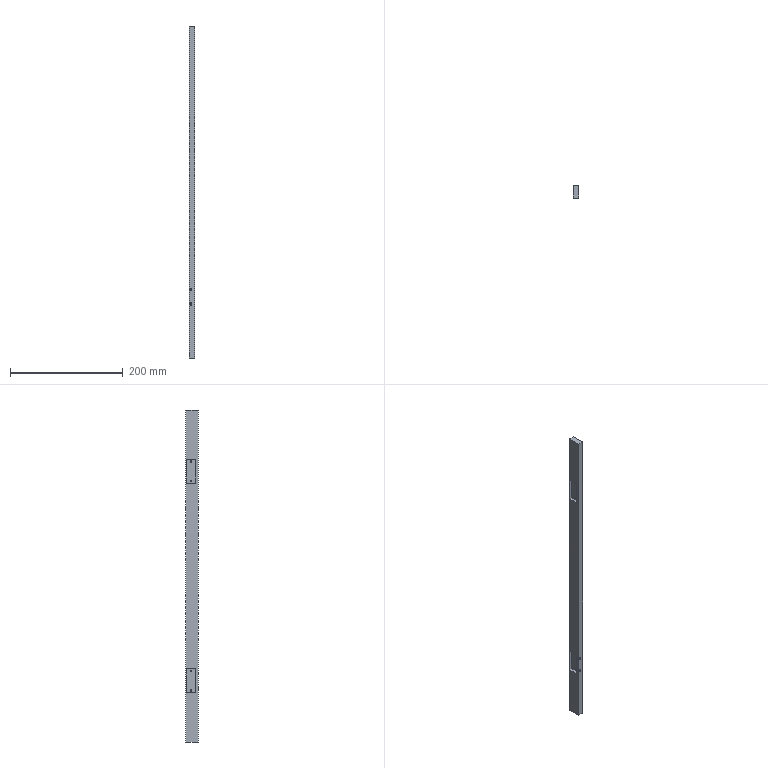Part | SolidWorks | features 3DProfileFeature 2, HoleWzd 2, MirrorPattern 2, Cut 1, Extrusion 1 | 1 solid | 46 faces | box 10 x 23 x 590 mm | volume 128132 mm3 | cylinder 24 | plane 22 | commonest cylinder face diameters 2.9 x8 5.5 x8 2.4 x4 4.4 x4
STEP:
#1=CARTESIAN_POINT('',(-2.5,2.4,-170.8));
#2=VERTEX_POINT('',#1);
#3=CARTESIAN_POINT('',(-2.5,2.4,-175.2));
#4=VERTEX_POINT('',#3);
#5=CARTESIAN_POINT('',(-2.5,2.4,-173.));
#6=DIRECTION('',(0.,-1.,0.));
#7=DIRECTION('',(0.,0.,-1.));
#8=AXIS2_PLACEMENT_3D('',#5,#6,#7);
#9=CIRCLE('',#8,2.2);
#10=EDGE_CURVE('',#2,#4,#9,.T.);
#11=ORIENTED_EDGE('',*,*,#10,.F.);
#12=CARTESIAN_POINT('',(-2.5,0.,-170.8));
#13=VERTEX_POINT('',#12);
#14=CARTESIAN_POINT('',(-2.5,0.,-170.8));
#15=DIRECTION('',(0.,-1.,0.));
#16=VECTOR('',#15,1000.);
#17=LINE('',#14,#16);
#18=EDGE_CURVE('',#2,#13,#17,.T.);
#19=ORIENTED_EDGE('',*,*,#18,.T.);
#20=CARTESIAN_POINT('',(-2.5,0.,-175.2));
#21=VERTEX_POINT('',#20);
#22=CARTESIAN_POINT('',(-2.5,0.,-173.));
#23=DIRECTION('',(0.,-1.,0.));
#24=DIRECTION('',(0.,0.,-1.));
#25=AXIS2_PLACEMENT_3D('',#22,#23,#24);
#26=CIRCLE('',#25,2.2);
#27=EDGE_CURVE('',#13,#21,#26,.T.);
#28=ORIENTED_EDGE('',*,*,#27,.T.);
#29=CARTESIAN_POINT('',(-2.5,0.,-175.2));
#30=DIRECTION('',(0.,-1.,0.));
#31=VECTOR('',#30,1000.);
#32=LINE('',#29,#31);
#33=EDGE_CURVE('',#4,#21,#32,.T.);
#34=ORIENTED_EDGE('',*,*,#33,.F.);
#35=EDGE_LOOP('',(#11,#19,#28,#34));
#36=FACE_OUTER_BOUND('',#35,.T.);
#37=CARTESIAN_POINT('',(-2.5,0.,-173.));
#38=DIRECTION('',(0.,-1.,0.));
#39=DIRECTION('',(0.,0.,-1.));
#40=AXIS2_PLACEMENT_3D('',#37,#38,#39);
#41=CYLINDRICAL_SURFACE('',#40,2.2);
#42=ADVANCED_FACE('',(#36),#41,.F.);
#43=CARTESIAN_POINT('',(-2.5,5.,-171.8));
#44=VERTEX_POINT('',#43);
#45=CARTESIAN_POINT('',(-2.5,5.,-174.2));
#46=VERTEX_POINT('',#45);
#47=CARTESIAN_POINT('',(-2.5,5.,-173.));
#48=DIRECTION('',(0.,-1.,0.));
#49=DIRECTION('',(0.,0.,-1.));
#50=AXIS2_PLACEMENT_3D('',#47,#48,#49);
#51=CIRCLE('',#50,1.2);
#52=EDGE_CURVE('',#44,#46,#51,.T.);
#53=ORIENTED_EDGE('',*,*,#52,.F.);
#54=CARTESIAN_POINT('',(-2.5,2.4,-171.8));
#55=VERTEX_POINT('',#54);
#56=CARTESIAN_POINT('',(-2.5,0.,-171.8));
#57=DIRECTION('',(0.,-1.,0.));
#58=VECTOR('',#57,1000.);
#59=LINE('',#56,#58);
#60=EDGE_CURVE('',#44,#55,#59,.T.);
#61=ORIENTED_EDGE('',*,*,#60,.T.);
#62=CARTESIAN_POINT('',(-2.5,2.4,-174.2));
#63=VERTEX_POINT('',#62);
#64=CARTESIAN_POINT('',(-2.5,2.4,-173.));
#65=DIRECTION('',(0.,-1.,0.));
#66=DIRECTION('',(0.,0.,-1.));
#67=AXIS2_PLACEMENT_3D('',#64,#65,#66);
#68=CIRCLE('',#67,1.2);
#69=EDGE_CURVE('',#55,#63,#68,.T.);
#70=ORIENTED_EDGE('',*,*,#69,.T.);
#71=CARTESIAN_POINT('',(-2.5,0.,-174.2));
#72=DIRECTION('',(0.,-1.,0.));
#73=VECTOR('',#72,1000.);
#74=LINE('',#71,#73);
#75=EDGE_CURVE('',#46,#63,#74,.T.);
#76=ORIENTED_EDGE('',*,*,#75,.F.);
#77=EDGE_LOOP('',(#53,#61,#70,#76));
#78=FACE_OUTER_BOUND('',#77,.T.);
#79=CARTESIAN_POINT('',(-2.5,0.,-173.));
#80=DIRECTION('',(0.,-1.,0.));
#81=DIRECTION('',(0.,0.,-1.));
#82=AXIS2_PLACEMENT_3D('',#79,#80,#81);
#83=CYLINDRICAL_SURFACE('',#82,1.2);
#84=ADVANCED_FACE('',(#78),#83,.F.);
#85=CARTESIAN_POINT('',(-2.5,2.4,-196.8));
#86=VERTEX_POINT('',#85);
#87=CARTESIAN_POINT('',(-2.5,2.4,-201.2));
#88=VERTEX_POINT('',#87);
#89=CARTESIAN_POINT('',(-2.5,2.4,-199.));
#90=DIRECTION('',(0.,-1.,0.));
#91=DIRECTION('',(0.,0.,-1.));
#92=AXIS2_PLACEMENT_3D('',#89,#90,#91);
#93=CIRCLE('',#92,2.2);
#94=EDGE_CURVE('',#86,#88,#93,.T.);
#95=ORIENTED_EDGE('',*,*,#94,.F.);
#96=CARTESIAN_POINT('',(-2.5,0.,-196.8));
#97=VERTEX_POINT('',#96);
#98=CARTESIAN_POINT('',(-2.5,0.,-196.8));
#99=DIRECTION('',(0.,-1.,0.));
#100=VECTOR('',#99,1000.);
#101=LINE('',#98,#100);
#102=EDGE_CURVE('',#86,#97,#101,.T.);
#103=ORIENTED_EDGE('',*,*,#102,.T.);
#104=CARTESIAN_POINT('',(-2.5,0.,-201.2));
#105=VERTEX_POINT('',#104);
#106=CARTESIAN_POINT('',(-2.5,0.,-199.));
#107=DIRECTION('',(0.,-1.,0.));
#108=DIRECTION('',(0.,0.,-1.));
#109=AXIS2_PLACEMENT_3D('',#106,#107,#108);
#110=CIRCLE('',#109,2.2);
#111=EDGE_CURVE('',#97,#105,#110,.T.);
#112=ORIENTED_EDGE('',*,*,#111,.T.);
#113=CARTESIAN_POINT('',(-2.5,0.,-201.2));
#114=DIRECTION('',(0.,-1.,0.));
#115=VECTOR('',#114,1000.);
#116=LINE('',#113,#115);
#117=EDGE_CURVE('',#88,#105,#116,.T.);
#118=ORIENTED_EDGE('',*,*,#117,.F.);
#119=EDGE_LOOP('',(#95,#103,#112,#118));
#120=FACE_OUTER_BOUND('',#119,.T.);
#121=CARTESIAN_POINT('',(-2.5,0.,-199.));
#122=DIRECTION('',(0.,-1.,0.));
#123=DIRECTION('',(0.,0.,-1.));
#124=AXIS2_PLACEMENT_3D('',#121,#122,#123);
#125=CYLINDRICAL_SURFACE('',#124,2.2);
#126=ADVANCED_FACE('',(#120),#125,.F.);
#127=CARTESIAN_POINT('',(-2.5,5.,-197.8));
#128=VERTEX_POINT('',#127);
#129=CARTESIAN_POINT('',(-2.5,5.,-200.2));
#130=VERTEX_POINT('',#129);
#131=CARTESIAN_POINT('',(-2.5,5.,-199.));
#132=DIRECTION('',(0.,-1.,0.));
#133=DIRECTION('',(0.,0.,-1.));
#134=AXIS2_PLACEMENT_3D('',#131,#132,#133);
#135=CIRCLE('',#134,1.2);
#136=EDGE_CURVE('',#128,#130,#135,.T.);
#137=ORIENTED_EDGE('',*,*,#136,.F.);
#138=CARTESIAN_POINT('',(-2.5,2.4,-197.8));
#139=VERTEX_POINT('',#138);
#140=CARTESIAN_POINT('',(-2.5,0.,-197.8));
#141=DIRECTION('',(0.,-1.,0.));
#142=VECTOR('',#141,1000.);
#143=LINE('',#140,#142);
#144=EDGE_CURVE('',#128,#139,#143,.T.);
#145=ORIENTED_EDGE('',*,*,#144,.T.);
#146=CARTESIAN_POINT('',(-2.5,2.4,-200.2));
#147=VERTEX_POINT('',#146);
#148=CARTESIAN_POINT('',(-2.5,2.4,-199.));
#149=DIRECTION('',(0.,-1.,0.));
#150=DIRECTION('',(0.,0.,-1.));
#151=AXIS2_PLACEMENT_3D('',#148,#149,#150);
#152=CIRCLE('',#151,1.2);
#153=EDGE_CURVE('',#139,#147,#152,.T.);
#154=ORIENTED_EDGE('',*,*,#153,.T.);
#155=CARTESIAN_POINT('',(-2.5,0.,-200.2));
#156=DIRECTION('',(0.,-1.,0.));
#157=VECTOR('',#156,1000.);
#158=LINE('',#155,#157);
#159=EDGE_CURVE('',#130,#147,#158,.T.);
#160=ORIENTED_EDGE('',*,*,#159,.F.);
#161=EDGE_LOOP('',(#137,#145,#154,#160));
#162=FACE_OUTER_BOUND('',#161,.T.);
#163=CARTESIAN_POINT('',(-2.5,0.,-199.));
#164=DIRECTION('',(0.,-1.,0.));
#165=DIRECTION('',(0.,0.,-1.));
#166=AXIS2_PLACEMENT_3D('',#163,#164,#165);
#167=CYLINDRICAL_SURFACE('',#166,1.2);
#168=ADVANCED_FACE('',(#162),#167,.F.);
#169=CARTESIAN_POINT('',(2.1,13.5,-200.25));
#170=VERTEX_POINT('',#169);
#171=CARTESIAN_POINT('',(2.1,13.5,-205.75));
#172=VERTEX_POINT('',#171);
#173=CARTESIAN_POINT('',(2.1,13.5,-203.));
#174=DIRECTION('',(1.,0.,0.));
#175=DIRECTION('',(0.,0.,-1.));
#176=AXIS2_PLACEMENT_3D('',#173,#174,#175);
#177=CIRCLE('',#176,2.75);
#178=EDGE_CURVE('',#170,#172,#177,.T.);
#179=ORIENTED_EDGE('',*,*,#178,.F.);
#180=CARTESIAN_POINT('',(5.,13.5,-200.25));
#181=VERTEX_POINT('',#180);
#182=CARTESIAN_POINT('',(5.,13.5,-200.25));
#183=DIRECTION('',(1.,0.,0.));
#184=VECTOR('',#183,1000.);
#185=LINE('',#182,#184);
#186=EDGE_CURVE('',#170,#181,#185,.T.);
#187=ORIENTED_EDGE('',*,*,#186,.T.);
#188=CARTESIAN_POINT('',(5.,13.5,-205.75));
#189=VERTEX_POINT('',#188);
#190=CARTESIAN_POINT('',(5.,13.5,-203.));
#191=DIRECTION('',(1.,0.,0.));
#192=DIRECTION('',(0.,0.,-1.));
#193=AXIS2_PLACEMENT_3D('',#190,#191,#192);
#194=CIRCLE('',#193,2.75);
#195=EDGE_CURVE('',#181,#189,#194,.T.);
#196=ORIENTED_EDGE('',*,*,#195,.T.);
#197=CARTESIAN_POINT('',(5.,13.5,-205.75));
#198=DIRECTION('',(1.,0.,0.));
#199=VECTOR('',#198,1000.);
#200=LINE('',#197,#199);
#201=EDGE_CURVE('',#172,#189,#200,.T.);
#202=ORIENTED_EDGE('',*,*,#201,.F.);
#203=EDGE_LOOP('',(#179,#187,#196,#202));
#204=FACE_OUTER_BOUND('',#203,.T.);
#205=CARTESIAN_POINT('',(5.,13.5,-203.));
#206=DIRECTION('',(1.,0.,0.));
#207=DIRECTION('',(0.,0.,-1.));
#208=AXIS2_PLACEMENT_3D('',#205,#206,#207);
#209=CYLINDRICAL_SURFACE('',#208,2.75);
#210=ADVANCED_FACE('',(#204),#209,.F.);
#211=CARTESIAN_POINT('',(0.,13.5,-204.45));
#212=VERTEX_POINT('',#211);
#213=CARTESIAN_POINT('',(0.,13.5,-201.55));
#214=VERTEX_POINT('',#213);
#215=CARTESIAN_POINT('',(0.,13.5,-203.));
#216=DIRECTION('',(-1.,0.,0.));
#217=DIRECTION('',(0.,0.,-1.));
#218=AXIS2_PLACEMENT_3D('',#215,#216,#217);
#219=CIRCLE('',#218,1.45);
#220=EDGE_CURVE('',#212,#214,#219,.T.);
#221=ORIENTED_EDGE('',*,*,#220,.T.);
#222=CARTESIAN_POINT('',(2.1,13.5,-201.55));
#223=VERTEX_POINT('',#222);
#224=CARTESIAN_POINT('',(5.,13.5,-201.55));
#225=DIRECTION('',(1.,0.,0.));
#226=VECTOR('',#225,1000.);
#227=LINE('',#224,#226);
#228=EDGE_CURVE('',#214,#223,#227,.T.);
#229=ORIENTED_EDGE('',*,*,#228,.T.);
#230=CARTESIAN_POINT('',(2.1,13.5,-204.45));
#231=VERTEX_POINT('',#230);
#232=CARTESIAN_POINT('',(2.1,13.5,-203.));
#233=DIRECTION('',(1.,0.,0.));
#234=DIRECTION('',(0.,0.,-1.));
#235=AXIS2_PLACEMENT_3D('',#232,#233,#234);
#236=CIRCLE('',#235,1.45);
#237=EDGE_CURVE('',#223,#231,#236,.T.);
#238=ORIENTED_EDGE('',*,*,#237,.T.);
#239=CARTESIAN_POINT('',(5.,13.5,-204.45));
#240=DIRECTION('',(1.,0.,0.));
#241=VECTOR('',#240,1000.);
#242=LINE('',#239,#241);
#243=EDGE_CURVE('',#212,#231,#242,.T.);
#244=ORIENTED_EDGE('',*,*,#243,.F.);
#245=EDGE_LOOP('',(#221,#229,#238,#244));
#246=FACE_OUTER_BOUND('',#245,.T.);
#247=CARTESIAN_POINT('',(5.,13.5,-203.));
#248=DIRECTION('',(1.,0.,0.));
#249=DIRECTION('',(0.,0.,-1.));
#250=AXIS2_PLACEMENT_3D('',#247,#248,#249);
#251=CYLINDRICAL_SURFACE('',#250,1.45);
#252=ADVANCED_FACE('',(#246),#251,.F.);
#253=CARTESIAN_POINT('',(2.1,13.5,-166.25));
#254=VERTEX_POINT('',#253);
#255=CARTESIAN_POINT('',(2.1,13.5,-171.75));
#256=VERTEX_POINT('',#255);
#257=CARTESIAN_POINT('',(2.1,13.5,-169.));
#258=DIRECTION('',(1.,0.,0.));
#259=DIRECTION('',(0.,0.,-1.));
#260=AXIS2_PLACEMENT_3D('',#257,#258,#259);
#261=CIRCLE('',#260,2.75);
#262=EDGE_CURVE('',#254,#256,#261,.T.);
#263=ORIENTED_EDGE('',*,*,#262,.F.);
#264=CARTESIAN_POINT('',(5.,13.5,-166.25));
#265=VERTEX_POINT('',#264);
#266=CARTESIAN_POINT('',(5.,13.5,-166.25));
#267=DIRECTION('',(1.,0.,0.));
#268=VECTOR('',#267,1000.);
#269=LINE('',#266,#268);
#270=EDGE_CURVE('',#254,#265,#269,.T.);
#271=ORIENTED_EDGE('',*,*,#270,.T.);
#272=CARTESIAN_POINT('',(5.,13.5,-171.75));
#273=VERTEX_POINT('',#272);
#274=CARTESIAN_POINT('',(5.,13.5,-169.));
#275=DIRECTION('',(1.,0.,0.));
#276=DIRECTION('',(0.,0.,-1.));
#277=AXIS2_PLACEMENT_3D('',#274,#275,#276);
#278=CIRCLE('',#277,2.75);
#279=EDGE_CURVE('',#265,#273,#278,.T.);
#280=ORIENTED_EDGE('',*,*,#279,.T.);
#281=CARTESIAN_POINT('',(5.,13.5,-171.75));
#282=DIRECTION('',(1.,0.,0.));
#283=VECTOR('',#282,1000.);
#284=LINE('',#281,#283);
#285=EDGE_CURVE('',#256,#273,#284,.T.);
#286=ORIENTED_EDGE('',*,*,#285,.F.);
#287=EDGE_LOOP('',(#263,#271,#280,#286));
#288=FACE_OUTER_BOUND('',#287,.T.);
#289=CARTESIAN_POINT('',(5.,13.5,-169.));
#290=DIRECTION('',(1.,0.,0.));
#291=DIRECTION('',(0.,0.,-1.));
#292=AXIS2_PLACEMENT_3D('',#289,#290,#291);
#293=CYLINDRICAL_SURFACE('',#292,2.75);
#294=ADVANCED_FACE('',(#288),#293,.F.);
#295=CARTESIAN_POINT('',(0.,13.5,-170.45));
#296=VERTEX_POINT('',#295);
#297=CARTESIAN_POINT('',(0.,13.5,-167.55));
#298=VERTEX_POINT('',#297);
#299=CARTESIAN_POINT('',(0.,13.5,-169.));
#300=DIRECTION('',(-1.,0.,0.));
#301=DIRECTION('',(0.,0.,-1.));
#302=AXIS2_PLACEMENT_3D('',#299,#300,#301);
#303=CIRCLE('',#302,1.45);
#304=EDGE_CURVE('',#296,#298,#303,.T.);
#305=ORIENTED_EDGE('',*,*,#304,.T.);
#306=CARTESIAN_POINT('',(2.1,13.5,-167.55));
#307=VERTEX_POINT('',#306);
#308=CARTESIAN_POINT('',(5.,13.5,-167.55));
#309=DIRECTION('',(1.,0.,0.));
#310=VECTOR('',#309,1000.);
#311=LINE('',#308,#310);
#312=EDGE_CURVE('',#298,#307,#311,.T.);
#313=ORIENTED_EDGE('',*,*,#312,.T.);
#314=CARTESIAN_POINT('',(2.1,13.5,-170.45));
#315=VERTEX_POINT('',#314);
#316=CARTESIAN_POINT('',(2.1,13.5,-169.));
#317=DIRECTION('',(1.,0.,0.));
#318=DIRECTION('',(0.,0.,-1.));
#319=AXIS2_PLACEMENT_3D('',#316,#317,#318);
#320=CIRCLE('',#319,1.45);
#321=EDGE_CURVE('',#307,#315,#320,.T.);
#322=ORIENTED_EDGE('',*,*,#321,.T.);
#323=CARTESIAN_POINT('',(5.,13.5,-170.45));
#324=DIRECTION('',(1.,0.,0.));
#325=VECTOR('',#324,1000.);
#326=LINE('',#323,#325);
#327=EDGE_CURVE('',#296,#315,#326,.T.);
#328=ORIENTED_EDGE('',*,*,#327,.F.);
#329=EDGE_LOOP('',(#305,#313,#322,#328));
#330=FACE_OUTER_BOUND('',#329,.T.);
#331=CARTESIAN_POINT('',(5.,13.5,-169.));
#332=DIRECTION('',(1.,0.,0.));
#333=DIRECTION('',(0.,0.,-1.));
#334=AXIS2_PLACEMENT_3D('',#331,#332,#333);
#335=CYLINDRICAL_SURFACE('',#334,1.45);
#336=ADVANCED_FACE('',(#330),#335,.F.);
#337=CARTESIAN_POINT('',(2.1,13.5,205.75));
#338=VERTEX_POINT('',#337);
#339=CARTESIAN_POINT('',(2.1,13.5,200.25));
#340=VERTEX_POINT('',#339);
#341=CARTESIAN_POINT('',(2.1,13.5,203.));
#342=DIRECTION('',(1.,0.,0.));
#343=DIRECTION('',(0.,0.,-1.));
#344=AXIS2_PLACEMENT_3D('',#341,#342,#343);
#345=CIRCLE('',#344,2.75);
#346=EDGE_CURVE('',#338,#340,#345,.T.);
#347=ORIENTED_EDGE('',*,*,#346,.F.);
#348=CARTESIAN_POINT('',(5.,13.5,205.75));
#349=VERTEX_POINT('',#348);
#350=CARTESIAN_POINT('',(5.,13.5,205.75));
#351=DIRECTION('',(1.,0.,0.));
#352=VECTOR('',#351,1000.);
#353=LINE('',#350,#352);
#354=EDGE_CURVE('',#338,#349,#353,.T.);
#355=ORIENTED_EDGE('',*,*,#354,.T.);
#356=CARTESIAN_POINT('',(5.,13.5,200.25));
#357=VERTEX_POINT('',#356);
#358=CARTESIAN_POINT('',(5.,13.5,203.));
#359=DIRECTION('',(1.,0.,0.));
#360=DIRECTION('',(0.,0.,-1.));
#361=AXIS2_PLACEMENT_3D('',#358,#359,#360);
#362=CIRCLE('',#361,2.75);
#363=EDGE_CURVE('',#349,#357,#362,.T.);
#364=ORIENTED_EDGE('',*,*,#363,.T.);
#365=CARTESIAN_POINT('',(5.,13.5,200.25));
#366=DIRECTION('',(1.,0.,0.));
#367=VECTOR('',#366,1000.);
#368=LINE('',#365,#367);
#369=EDGE_CURVE('',#340,#357,#368,.T.);
#370=ORIENTED_EDGE('',*,*,#369,.F.);
#371=EDGE_LOOP('',(#347,#355,#364,#370));
#372=FACE_OUTER_BOUND('',#371,.T.);
#373=CARTESIAN_POINT('',(5.,13.5,203.));
#374=DIRECTION('',(1.,0.,0.));
#375=DIRECTION('',(0.,0.,-1.));
#376=AXIS2_PLACEMENT_3D('',#373,#374,#375);
#377=CYLINDRICAL_SURFACE('',#376,2.75);
#378=ADVANCED_FACE('',(#372),#377,.F.);
#379=CARTESIAN_POINT('',(2.1,13.5,171.75));
#380=VERTEX_POINT('',#379);
#381=CARTESIAN_POINT('',(2.1,13.5,166.25));
#382=VERTEX_POINT('',#381);
#383=CARTESIAN_POINT('',(2.1,13.5,169.));
#384=DIRECTION('',(1.,0.,0.));
#385=DIRECTION('',(0.,0.,-1.));
#386=AXIS2_PLACEMENT_3D('',#383,#384,#385);
#387=CIRCLE('',#386,2.75);
#388=EDGE_CURVE('',#380,#382,#387,.T.);
#389=ORIENTED_EDGE('',*,*,#388,.F.);
#390=CARTESIAN_POINT('',(5.,13.5,171.75));
#391=VERTEX_POINT('',#390);
#392=CARTESIAN_POINT('',(5.,13.5,171.75));
#393=DIRECTION('',(1.,0.,0.));
#394=VECTOR('',#393,1000.);
#395=LINE('',#392,#394);
#396=EDGE_CURVE('',#380,#391,#395,.T.);
#397=ORIENTED_EDGE('',*,*,#396,.T.);
#398=CARTESIAN_POINT('',(5.,13.5,166.25));
#399=VERTEX_POINT('',#398);
#400=CARTESIAN_POINT('',(5.,13.5,169.));
#401=DIRECTION('',(1.,0.,0.));
#402=DIRECTION('',(0.,0.,-1.));
#403=AXIS2_PLACEMENT_3D('',#400,#401,#402);
#404=CIRCLE('',#403,2.75);
#405=EDGE_CURVE('',#391,#399,#404,.T.);
#406=ORIENTED_EDGE('',*,*,#405,.T.);
#407=CARTESIAN_POINT('',(5.,13.5,166.25));
#408=DIRECTION('',(1.,0.,0.));
#409=VECTOR('',#408,1000.);
#410=LINE('',#407,#409);
#411=EDGE_CURVE('',#382,#399,#410,.T.);
#412=ORIENTED_EDGE('',*,*,#411,.F.);
#413=EDGE_LOOP('',(#389,#397,#406,#412));
#414=FACE_OUTER_BOUND('',#413,.T.);
#415=CARTESIAN_POINT('',(5.,13.5,169.));
#416=DIRECTION('',(1.,0.,0.));
#417=DIRECTION('',(0.,0.,-1.));
#418=AXIS2_PLACEMENT_3D('',#415,#416,#417);
#419=CYLINDRICAL_SURFACE('',#418,2.75);
#420=ADVANCED_FACE('',(#414),#419,.F.);
#421=CARTESIAN_POINT('',(0.,13.5,204.45));
#422=VERTEX_POINT('',#421);
#423=CARTESIAN_POINT('',(0.,13.5,201.55));
#424=VERTEX_POINT('',#423);
#425=CARTESIAN_POINT('',(0.,13.5,203.));
#426=DIRECTION('',(1.,0.,0.));
#427=DIRECTION('',(0.,0.,1.));
#428=AXIS2_PLACEMENT_3D('',#425,#426,#427);
#429=CIRCLE('',#428,1.45);
#430=EDGE_CURVE('',#422,#424,#429,.T.);
#431=ORIENTED_EDGE('',*,*,#430,.F.);
#432=CARTESIAN_POINT('',(2.1,13.5,204.45));
#433=VERTEX_POINT('',#432);
#434=CARTESIAN_POINT('',(5.,13.5,204.45));
#435=DIRECTION('',(1.,0.,0.));
#436=VECTOR('',#435,1000.);
#437=LINE('',#434,#436);
#438=EDGE_CURVE('',#422,#433,#437,.T.);
#439=ORIENTED_EDGE('',*,*,#438,.T.);
#440=CARTESIAN_POINT('',(2.1,13.5,201.55));
#441=VERTEX_POINT('',#440);
#442=CARTESIAN_POINT('',(2.1,13.5,203.));
#443=DIRECTION('',(1.,0.,0.));
#444=DIRECTION('',(0.,0.,-1.));
#445=AXIS2_PLACEMENT_3D('',#442,#443,#444);
#446=CIRCLE('',#445,1.45);
#447=EDGE_CURVE('',#433,#441,#446,.T.);
#448=ORIENTED_EDGE('',*,*,#447,.T.);
#449=CARTESIAN_POINT('',(5.,13.5,201.55));
#450=DIRECTION('',(1.,0.,0.));
#451=VECTOR('',#450,1000.);
#452=LINE('',#449,#451);
#453=EDGE_CURVE('',#424,#441,#452,.T.);
#454=ORIENTED_EDGE('',*,*,#453,.F.);
#455=EDGE_LOOP('',(#431,#439,#448,#454));
#456=FACE_OUTER_BOUND('',#455,.T.);
#457=CARTESIAN_POINT('',(5.,13.5,203.));
#458=DIRECTION('',(1.,0.,0.));
#459=DIRECTION('',(0.,0.,-1.));
#460=AXIS2_PLACEMENT_3D('',#457,#458,#459);
#461=CYLINDRICAL_SURFACE('',#460,1.45);
#462=ADVANCED_FACE('',(#456),#461,.F.);
#463=CARTESIAN_POINT('',(0.,13.5,170.45));
#464=VERTEX_POINT('',#463);
#465=CARTESIAN_POINT('',(0.,13.5,167.55));
#466=VERTEX_POINT('',#465);
#467=CARTESIAN_POINT('',(0.,13.5,169.));
#468=DIRECTION('',(1.,0.,0.));
#469=DIRECTION('',(0.,0.,1.));
#470=AXIS2_PLACEMENT_3D('',#467,#468,#469);
#471=CIRCLE('',#470,1.45);
#472=EDGE_CURVE('',#464,#466,#471,.T.);
#473=ORIENTED_EDGE('',*,*,#472,.F.);
#474=CARTESIAN_POINT('',(2.1,13.5,170.45));
#475=VERTEX_POINT('',#474);
#476=CARTESIAN_POINT('',(5.,13.5,170.45));
#477=DIRECTION('',(1.,0.,0.));
#478=VECTOR('',#477,1000.);
#479=LINE('',#476,#478);
#480=EDGE_CURVE('',#464,#475,#479,.T.);
#481=ORIENTED_EDGE('',*,*,#480,.T.);
#482=CARTESIAN_POINT('',(2.1,13.5,167.55));
#483=VERTEX_POINT('',#482);
#484=CARTESIAN_POINT('',(2.1,13.5,169.));
#485=DIRECTION('',(1.,0.,0.));
#486=DIRECTION('',(0.,0.,-1.));
#487=AXIS2_PLACEMENT_3D('',#484,#485,#486);
#488=CIRCLE('',#487,1.45);
#489=EDGE_CURVE('',#475,#483,#488,.T.);
#490=ORIENTED_EDGE('',*,*,#489,.T.);
#491=CARTESIAN_POINT('',(5.,13.5,167.55));
#492=DIRECTION('',(1.,0.,0.));
#493=VECTOR('',#492,1000.);
#494=LINE('',#491,#493);
#495=EDGE_CURVE('',#466,#483,#494,.T.);
#496=ORIENTED_EDGE('',*,*,#495,.F.);
#497=EDGE_LOOP('',(#473,#481,#490,#496));
#498=FACE_OUTER_BOUND('',#497,.T.);
#499=CARTESIAN_POINT('',(5.,13.5,169.));
#500=DIRECTION('',(1.,0.,0.));
#501=DIRECTION('',(0.,0.,-1.));
#502=AXIS2_PLACEMENT_3D('',#499,#500,#501);
#503=CYLINDRICAL_SURFACE('',#502,1.45);
#504=ADVANCED_FACE('',(#498),#503,.F.);
#505=ORIENTED_EDGE('',*,*,#480,.F.);
#506=CARTESIAN_POINT('',(0.,13.5,169.));
#507=DIRECTION('',(1.,0.,0.));
#508=DIRECTION('',(0.,0.,1.));
#509=AXIS2_PLACEMENT_3D('',#506,#507,#508);
#510=CIRCLE('',#509,1.45);
#511=EDGE_CURVE('',#466,#464,#510,.T.);
#512=ORIENTED_EDGE('',*,*,#511,.F.);
#513=ORIENTED_EDGE('',*,*,#495,.T.);
#514=CARTESIAN_POINT('',(2.1,13.5,169.));
#515=DIRECTION('',(1.,0.,0.));
#516=DIRECTION('',(0.,0.,-1.));
#517=AXIS2_PLACEMENT_3D('',#514,#515,#516);
#518=CIRCLE('',#517,1.45);
#519=EDGE_CURVE('',#483,#475,#518,.T.);
#520=ORIENTED_EDGE('',*,*,#519,.T.);
#521=EDGE_LOOP('',(#505,#512,#513,#520));
#522=FACE_OUTER_BOUND('',#521,.T.);
#523=CARTESIAN_POINT('',(5.,13.5,169.));
#524=DIRECTION('',(1.,0.,0.));
#525=DIRECTION('',(0.,0.,-1.));
#526=AXIS2_PLACEMENT_3D('',#523,#524,#525);
#527=CYLINDRICAL_SURFACE('',#526,1.45);
#528=ADVANCED_FACE('',(#522),#527,.F.);
#529=ORIENTED_EDGE('',*,*,#438,.F.);
#530=CARTESIAN_POINT('',(0.,13.5,203.));
#531=DIRECTION('',(1.,0.,0.));
#532=DIRECTION('',(0.,0.,1.));
#533=AXIS2_PLACEMENT_3D('',#530,#531,#532);
#534=CIRCLE('',#533,1.45);
#535=EDGE_CURVE('',#424,#422,#534,.T.);
#536=ORIENTED_EDGE('',*,*,#535,.F.);
#537=ORIENTED_EDGE('',*,*,#453,.T.);
#538=CARTESIAN_POINT('',(2.1,13.5,203.));
#539=DIRECTION('',(1.,0.,0.));
#540=DIRECTION('',(0.,0.,-1.));
#541=AXIS2_PLACEMENT_3D('',#538,#539,#540);
#542=CIRCLE('',#541,1.45);
#543=EDGE_CURVE('',#441,#433,#542,.T.);
#544=ORIENTED_EDGE('',*,*,#543,.T.);
#545=EDGE_LOOP('',(#529,#536,#537,#544));
#546=FACE_OUTER_BOUND('',#545,.T.);
#547=CARTESIAN_POINT('',(5.,13.5,203.));
#548=DIRECTION('',(1.,0.,0.));
#549=DIRECTION('',(0.,0.,-1.));
#550=AXIS2_PLACEMENT_3D('',#547,#548,#549);
#551=CYLINDRICAL_SURFACE('',#550,1.45);
#552=ADVANCED_FACE('',(#546),#551,.F.);
#553=CARTESIAN_POINT('',(-5.,5.,207.));
#554=VERTEX_POINT('',#553);
#555=CARTESIAN_POINT('',(-5.,22.,207.));
#556=VERTEX_POINT('',#555);
#557=CARTESIAN_POINT('',(-5.,5.,207.));
#558=DIRECTION('',(0.,1.,0.));
#559=VECTOR('',#558,1000.);
#560=LINE('',#557,#559);
#561=EDGE_CURVE('',#554,#556,#560,.T.);
#562=ORIENTED_EDGE('',*,*,#561,.F.);
#563=CARTESIAN_POINT('',(-5.,5.,165.));
#564=VERTEX_POINT('',#563);
#565=CARTESIAN_POINT('',(-5.,5.,207.));
#566=DIRECTION('',(0.,0.,-1.));
#567=VECTOR('',#566,1000.);
#568=LINE('',#565,#567);
#569=EDGE_CURVE('',#554,#564,#568,.T.);
#570=ORIENTED_EDGE('',*,*,#569,.T.);
#571=CARTESIAN_POINT('',(-5.,22.,165.));
#572=VERTEX_POINT('',#571);
#573=CARTESIAN_POINT('',(-5.,5.,165.));
#574=DIRECTION('',(0.,1.,0.));
#575=VECTOR('',#574,1000.);
#576=LINE('',#573,#575);
#577=EDGE_CURVE('',#564,#572,#576,.T.);
#578=ORIENTED_EDGE('',*,*,#577,.T.);
#579=CARTESIAN_POINT('',(-5.,22.,207.));
#580=DIRECTION('',(0.,0.,-1.));
#581=VECTOR('',#580,1000.);
#582=LINE('',#579,#581);
#583=EDGE_CURVE('',#556,#572,#582,.T.);
#584=ORIENTED_EDGE('',*,*,#583,.F.);
#585=EDGE_LOOP('',(#562,#570,#578,#584));
#586=FACE_BOUND('',#585,.T.);
#587=CARTESIAN_POINT('',(-5.,5.,-165.));
#588=VERTEX_POINT('',#587);
#589=CARTESIAN_POINT('',(-5.,22.,-165.));
#590=VERTEX_POINT('',#589);
#591=CARTESIAN_POINT('',(-5.,5.,-165.));
#592=DIRECTION('',(0.,1.,0.));
#593=VECTOR('',#592,1000.);
#594=LINE('',#591,#593);
#595=EDGE_CURVE('',#588,#590,#594,.T.);
#596=ORIENTED_EDGE('',*,*,#595,.F.);
#597=CARTESIAN_POINT('',(-5.,5.,-207.));
#598=VERTEX_POINT('',#597);
#599=CARTESIAN_POINT('',(-5.,5.,-207.));
#600=DIRECTION('',(0.,0.,1.));
#601=VECTOR('',#600,1000.);
#602=LINE('',#599,#601);
#603=EDGE_CURVE('',#598,#588,#602,.T.);
#604=ORIENTED_EDGE('',*,*,#603,.F.);
#605=CARTESIAN_POINT('',(-5.,22.,-207.));
#606=VERTEX_POINT('',#605);
#607=CARTESIAN_POINT('',(-5.,5.,-207.));
#608=DIRECTION('',(0.,1.,0.));
#609=VECTOR('',#608,1000.);
#610=LINE('',#607,#609);
#611=EDGE_CURVE('',#598,#606,#610,.T.);
#612=ORIENTED_EDGE('',*,*,#611,.T.);
#613=CARTESIAN_POINT('',(-5.,22.,-207.));
#614=DIRECTION('',(0.,0.,1.));
#615=VECTOR('',#614,1000.);
#616=LINE('',#613,#615);
#617=EDGE_CURVE('',#606,#590,#616,.T.);
#618=ORIENTED_EDGE('',*,*,#617,.T.);
#619=EDGE_LOOP('',(#596,#604,#612,#618));
#620=FACE_BOUND('',#619,.T.);
#621=CARTESIAN_POINT('',(-5.,0.,-295.));
#622=VERTEX_POINT('',#621);
#623=CARTESIAN_POINT('',(-5.,0.,295.));
#624=VERTEX_POINT('',#623);
#625=CARTESIAN_POINT('',(-5.,0.,-295.));
#626=DIRECTION('',(0.,0.,1.));
#627=VECTOR('',#626,1000.);
#628=LINE('',#625,#627);
#629=EDGE_CURVE('',#622,#624,#628,.T.);
#630=ORIENTED_EDGE('',*,*,#629,.T.);
#631=CARTESIAN_POINT('',(-5.,23.,295.));
#632=VERTEX_POINT('',#631);
#633=CARTESIAN_POINT('',(-5.,23.,295.));
#634=DIRECTION('',(0.,-1.,0.));
#635=VECTOR('',#634,1000.);
#636=LINE('',#633,#635);
#637=EDGE_CURVE('',#632,#624,#636,.T.);
#638=ORIENTED_EDGE('',*,*,#637,.F.);
#639=CARTESIAN_POINT('',(-5.,23.,-295.));
#640=VERTEX_POINT('',#639);
#641=CARTESIAN_POINT('',(-5.,23.,-295.));
#642=DIRECTION('',(0.,0.,1.));
#643=VECTOR('',#642,1000.);
#644=LINE('',#641,#643);
#645=EDGE_CURVE('',#640,#632,#644,.T.);
#646=ORIENTED_EDGE('',*,*,#645,.F.);
#647=CARTESIAN_POINT('',(-5.,23.,-295.));
#648=DIRECTION('',(0.,-1.,0.));
#649=VECTOR('',#648,1000.);
#650=LINE('',#647,#649);
#651=EDGE_CURVE('',#640,#622,#650,.T.);
#652=ORIENTED_EDGE('',*,*,#651,.T.);
#653=EDGE_LOOP('',(#630,#638,#646,#652));
#654=FACE_OUTER_BOUND('',#653,.T.);
#655=CARTESIAN_POINT('',(-5.,23.,-295.));
#656=DIRECTION('',(1.,0.,0.));
#657=DIRECTION('',(0.,0.,-1.));
#658=AXIS2_PLACEMENT_3D('',#655,#656,#657);
#659=PLANE('',#658);
#660=ADVANCED_FACE('',(#586,#620,#654),#659,.F.);
#661=CARTESIAN_POINT('',(5.,0.,295.));
#662=VERTEX_POINT('',#661);
#663=CARTESIAN_POINT('',(5.,0.,295.));
#664=DIRECTION('',(1.,0.,0.));
#665=VECTOR('',#664,1000.);
#666=LINE('',#663,#665);
#667=EDGE_CURVE('',#624,#662,#666,.T.);
#668=ORIENTED_EDGE('',*,*,#667,.T.);
#669=CARTESIAN_POINT('',(5.,23.,295.));
#670=VERTEX_POINT('',#669);
#671=CARTESIAN_POINT('',(5.,23.,295.));
#672=DIRECTION('',(0.,-1.,0.));
#673=VECTOR('',#672,1000.);
#674=LINE('',#671,#673);
#675=EDGE_CURVE('',#670,#662,#674,.T.);
#676=ORIENTED_EDGE('',*,*,#675,.F.);
#677=CARTESIAN_POINT('',(5.,23.,295.));
#678=DIRECTION('',(1.,0.,0.));
#679=VECTOR('',#678,1000.);
#680=LINE('',#677,#679);
#681=EDGE_CURVE('',#632,#670,#680,.T.);
#682=ORIENTED_EDGE('',*,*,#681,.F.);
#683=ORIENTED_EDGE('',*,*,#637,.T.);
#684=EDGE_LOOP('',(#668,#676,#682,#683));
#685=FACE_OUTER_BOUND('',#684,.T.);
#686=CARTESIAN_POINT('',(5.,23.,295.));
#687=DIRECTION('',(0.,0.,-1.));
#688=DIRECTION('',(-1.,0.,0.));
#689=AXIS2_PLACEMENT_3D('',#686,#687,#688);
#690=PLANE('',#689);
#691=ADVANCED_FACE('',(#685),#690,.F.);
#692=CARTESIAN_POINT('',(5.,13.5,-203.));
#693=DIRECTION('',(1.,0.,0.));
#694=DIRECTION('',(0.,0.,-1.));
#695=AXIS2_PLACEMENT_3D('',#692,#693,#694);
#696=CIRCLE('',#695,2.75);
#697=EDGE_CURVE('',#189,#181,#696,.T.);
#698=ORIENTED_EDGE('',*,*,#697,.F.);
#699=ORIENTED_EDGE('',*,*,#195,.F.);
#700=EDGE_LOOP('',(#698,#699));
#701=FACE_BOUND('',#700,.T.);
#702=CARTESIAN_POINT('',(5.,13.5,-169.));
#703=DIRECTION('',(1.,0.,0.));
#704=DIRECTION('',(0.,0.,-1.));
#705=AXIS2_PLACEMENT_3D('',#702,#703,#704);
#706=CIRCLE('',#705,2.75);
#707=EDGE_CURVE('',#273,#265,#706,.T.);
#708=ORIENTED_EDGE('',*,*,#707,.F.);
#709=ORIENTED_EDGE('',*,*,#279,.F.);
#710=EDGE_LOOP('',(#708,#709));
#711=FACE_BOUND('',#710,.T.);
#712=CARTESIAN_POINT('',(5.,13.5,203.));
#713=DIRECTION('',(1.,0.,0.));
#714=DIRECTION('',(0.,0.,-1.));
#715=AXIS2_PLACEMENT_3D('',#712,#713,#714);
#716=CIRCLE('',#715,2.75);
#717=EDGE_CURVE('',#357,#349,#716,.T.);
#718=ORIENTED_EDGE('',*,*,#717,.F.);
#719=ORIENTED_EDGE('',*,*,#363,.F.);
#720=EDGE_LOOP('',(#718,#719));
#721=FACE_BOUND('',#720,.T.);
#722=CARTESIAN_POINT('',(5.,13.5,169.));
#723=DIRECTION('',(1.,0.,0.));
#724=DIRECTION('',(0.,0.,-1.));
#725=AXIS2_PLACEMENT_3D('',#722,#723,#724);
#726=CIRCLE('',#725,2.75);
#727=EDGE_CURVE('',#399,#391,#726,.T.);
#728=ORIENTED_EDGE('',*,*,#727,.F.);
#729=ORIENTED_EDGE('',*,*,#405,.F.);
#730=EDGE_LOOP('',(#728,#729));
#731=FACE_BOUND('',#730,.T.);
#732=CARTESIAN_POINT('',(5.,0.,-295.));
#733=VERTEX_POINT('',#732);
#734=CARTESIAN_POINT('',(5.,0.,-295.));
#735=DIRECTION('',(0.,0.,-1.));
#736=VECTOR('',#735,1000.);
#737=LINE('',#734,#736);
#738=EDGE_CURVE('',#662,#733,#737,.T.);
#739=ORIENTED_EDGE('',*,*,#738,.T.);
#740=CARTESIAN_POINT('',(5.,23.,-295.));
#741=VERTEX_POINT('',#740);
#742=CARTESIAN_POINT('',(5.,23.,-295.));
#743=DIRECTION('',(0.,-1.,0.));
#744=VECTOR('',#743,1000.);
#745=LINE('',#742,#744);
#746=EDGE_CURVE('',#741,#733,#745,.T.);
#747=ORIENTED_EDGE('',*,*,#746,.F.);
#748=CARTESIAN_POINT('',(5.,23.,-295.));
#749=DIRECTION('',(0.,0.,-1.));
#750=VECTOR('',#749,1000.);
#751=LINE('',#748,#750);
#752=EDGE_CURVE('',#670,#741,#751,.T.);
#753=ORIENTED_EDGE('',*,*,#752,.F.);
#754=ORIENTED_EDGE('',*,*,#675,.T.);
#755=EDGE_LOOP('',(#739,#747,#753,#754));
#756=FACE_OUTER_BOUND('',#755,.T.);
#757=CARTESIAN_POINT('',(5.,23.,-295.));
#758=DIRECTION('',(-1.,0.,0.));
#759=DIRECTION('',(0.,0.,1.));
#760=AXIS2_PLACEMENT_3D('',#757,#758,#759);
#761=PLANE('',#760);
#762=ADVANCED_FACE('',(#701,#711,#721,#731,#756),#761,.F.);
#763=CARTESIAN_POINT('',(5.,0.,-295.));
#764=DIRECTION('',(-1.,0.,0.));
#765=VECTOR('',#764,1000.);
#766=LINE('',#763,#765);
#767=EDGE_CURVE('',#733,#622,#766,.T.);
#768=ORIENTED_EDGE('',*,*,#767,.T.);
#769=ORIENTED_EDGE('',*,*,#651,.F.);
#770=CARTESIAN_POINT('',(5.,23.,-295.));
#771=DIRECTION('',(-1.,0.,0.));
#772=VECTOR('',#771,1000.);
#773=LINE('',#770,#772);
#774=EDGE_CURVE('',#741,#640,#773,.T.);
#775=ORIENTED_EDGE('',*,*,#774,.F.);
#776=ORIENTED_EDGE('',*,*,#746,.T.);
#777=EDGE_LOOP('',(#768,#769,#775,#776));
#778=FACE_OUTER_BOUND('',#777,.T.);
#779=CARTESIAN_POINT('',(5.,23.,-295.));
#780=DIRECTION('',(0.,0.,1.));
#781=DIRECTION('',(1.,0.,0.));
#782=AXIS2_PLACEMENT_3D('',#779,#780,#781);
#783=PLANE('',#782);
#784=ADVANCED_FACE('',(#778),#783,.F.);
#785=ORIENTED_EDGE('',*,*,#645,.T.);
#786=ORIENTED_EDGE('',*,*,#681,.T.);
#787=ORIENTED_EDGE('',*,*,#752,.T.);
#788=ORIENTED_EDGE('',*,*,#774,.T.);
#789=EDGE_LOOP('',(#785,#786,#787,#788));
#790=FACE_OUTER_BOUND('',#789,.T.);
#791=CARTESIAN_POINT('',(0.,23.,0.));
#792=DIRECTION('',(0.,-1.,0.));
#793=DIRECTION('',(0.,0.,-1.));
#794=AXIS2_PLACEMENT_3D('',#791,#792,#793);
#795=PLANE('',#794);
#796=ADVANCED_FACE('',(#790),#795,.F.);
#797=CARTESIAN_POINT('',(-2.5,0.,-173.));
#798=DIRECTION('',(0.,-1.,0.));
#799=DIRECTION('',(0.,0.,-1.));
#800=AXIS2_PLACEMENT_3D('',#797,#798,#799);
#801=CIRCLE('',#800,2.2);
#802=EDGE_CURVE('',#21,#13,#801,.T.);
#803=ORIENTED_EDGE('',*,*,#802,.F.);
#804=ORIENTED_EDGE('',*,*,#27,.F.);
#805=EDGE_LOOP('',(#803,#804));
#806=FACE_BOUND('',#805,.T.);
#807=CARTESIAN_POINT('',(-2.5,0.,-199.));
#808=DIRECTION('',(0.,-1.,0.));
#809=DIRECTION('',(0.,0.,-1.));
#810=AXIS2_PLACEMENT_3D('',#807,#808,#809);
#811=CIRCLE('',#810,2.2);
#812=EDGE_CURVE('',#105,#97,#811,.T.);
#813=ORIENTED_EDGE('',*,*,#812,.F.);
#814=ORIENTED_EDGE('',*,*,#111,.F.);
#815=EDGE_LOOP('',(#813,#814));
#816=FACE_BOUND('',#815,.T.);
#817=ORIENTED_EDGE('',*,*,#629,.F.);
#818=ORIENTED_EDGE('',*,*,#767,.F.);
#819=ORIENTED_EDGE('',*,*,#738,.F.);
#820=ORIENTED_EDGE('',*,*,#667,.F.);
#821=EDGE_LOOP('',(#817,#818,#819,#820));
#822=FACE_OUTER_BOUND('',#821,.T.);
#823=CARTESIAN_POINT('',(0.,0.,0.));
#824=DIRECTION('',(0.,-1.,0.));
#825=DIRECTION('',(0.,0.,-1.));
#826=AXIS2_PLACEMENT_3D('',#823,#824,#825);
#827=PLANE('',#826);
#828=ADVANCED_FACE('',(#806,#816,#822),#827,.T.);
#829=ORIENTED_EDGE('',*,*,#519,.F.);
#830=ORIENTED_EDGE('',*,*,#489,.F.);
#831=EDGE_LOOP('',(#829,#830));
#832=FACE_BOUND('',#831,.T.);
#833=CARTESIAN_POINT('',(2.1,13.5,169.));
#834=DIRECTION('',(1.,0.,0.));
#835=DIRECTION('',(0.,0.,-1.));
#836=AXIS2_PLACEMENT_3D('',#833,#834,#835);
#837=CIRCLE('',#836,2.75);
#838=EDGE_CURVE('',#382,#380,#837,.T.);
#839=ORIENTED_EDGE('',*,*,#838,.T.);
#840=ORIENTED_EDGE('',*,*,#388,.T.);
#841=EDGE_LOOP('',(#839,#840));
#842=FACE_OUTER_BOUND('',#841,.T.);
#843=CARTESIAN_POINT('',(2.1,14.95,169.));
#844=DIRECTION('',(-1.,0.,0.));
#845=DIRECTION('',(0.,0.,1.));
#846=AXIS2_PLACEMENT_3D('',#843,#844,#845);
#847=PLANE('',#846);
#848=ADVANCED_FACE('',(#832,#842),#847,.F.);
#849=ORIENTED_EDGE('',*,*,#396,.F.);
#850=ORIENTED_EDGE('',*,*,#838,.F.);
#851=ORIENTED_EDGE('',*,*,#411,.T.);
#852=ORIENTED_EDGE('',*,*,#727,.T.);
#853=EDGE_LOOP('',(#849,#850,#851,#852));
#854=FACE_OUTER_BOUND('',#853,.T.);
#855=CARTESIAN_POINT('',(5.,13.5,169.));
#856=DIRECTION('',(1.,0.,0.));
#857=DIRECTION('',(0.,0.,-1.));
#858=AXIS2_PLACEMENT_3D('',#855,#856,#857);
#859=CYLINDRICAL_SURFACE('',#858,2.75);
#860=ADVANCED_FACE('',(#854),#859,.F.);
#861=ORIENTED_EDGE('',*,*,#543,.F.);
#862=ORIENTED_EDGE('',*,*,#447,.F.);
#863=EDGE_LOOP('',(#861,#862));
#864=FACE_BOUND('',#863,.T.);
#865=CARTESIAN_POINT('',(2.1,13.5,203.));
#866=DIRECTION('',(1.,0.,0.));
#867=DIRECTION('',(0.,0.,-1.));
#868=AXIS2_PLACEMENT_3D('',#865,#866,#867);
#869=CIRCLE('',#868,2.75);
#870=EDGE_CURVE('',#340,#338,#869,.T.);
#871=ORIENTED_EDGE('',*,*,#870,.T.);
#872=ORIENTED_EDGE('',*,*,#346,.T.);
#873=EDGE_LOOP('',(#871,#872));
#874=FACE_OUTER_BOUND('',#873,.T.);
#875=CARTESIAN_POINT('',(2.1,14.95,203.));
#876=DIRECTION('',(-1.,0.,0.));
#877=DIRECTION('',(0.,0.,1.));
#878=AXIS2_PLACEMENT_3D('',#875,#876,#877);
#879=PLANE('',#878);
#880=ADVANCED_FACE('',(#864,#874),#879,.F.);
#881=ORIENTED_EDGE('',*,*,#354,.F.);
#882=ORIENTED_EDGE('',*,*,#870,.F.);
#883=ORIENTED_EDGE('',*,*,#369,.T.);
#884=ORIENTED_EDGE('',*,*,#717,.T.);
#885=EDGE_LOOP('',(#881,#882,#883,#884));
#886=FACE_OUTER_BOUND('',#885,.T.);
#887=CARTESIAN_POINT('',(5.,13.5,203.));
#888=DIRECTION('',(1.,0.,0.));
#889=DIRECTION('',(0.,0.,-1.));
#890=AXIS2_PLACEMENT_3D('',#887,#888,#889);
#891=CYLINDRICAL_SURFACE('',#890,2.75);
#892=ADVANCED_FACE('',(#886),#891,.F.);
#893=ORIENTED_EDGE('',*,*,#312,.F.);
#894=CARTESIAN_POINT('',(0.,13.5,-169.));
#895=DIRECTION('',(-1.,0.,0.));
#896=DIRECTION('',(0.,0.,-1.));
#897=AXIS2_PLACEMENT_3D('',#894,#895,#896);
#898=CIRCLE('',#897,1.45);
#899=EDGE_CURVE('',#298,#296,#898,.T.);
#900=ORIENTED_EDGE('',*,*,#899,.T.);
#901=ORIENTED_EDGE('',*,*,#327,.T.);
#902=CARTESIAN_POINT('',(2.1,13.5,-169.));
#903=DIRECTION('',(1.,0.,0.));
#904=DIRECTION('',(0.,0.,-1.));
#905=AXIS2_PLACEMENT_3D('',#902,#903,#904);
#906=CIRCLE('',#905,1.45);
#907=EDGE_CURVE('',#315,#307,#906,.T.);
#908=ORIENTED_EDGE('',*,*,#907,.T.);
#909=EDGE_LOOP('',(#893,#900,#901,#908));
#910=FACE_OUTER_BOUND('',#909,.T.);
#911=CARTESIAN_POINT('',(5.,13.5,-169.));
#912=DIRECTION('',(1.,0.,0.));
#913=DIRECTION('',(0.,0.,-1.));
#914=AXIS2_PLACEMENT_3D('',#911,#912,#913);
#915=CYLINDRICAL_SURFACE('',#914,1.45);
#916=ADVANCED_FACE('',(#910),#915,.F.);
#917=ORIENTED_EDGE('',*,*,#907,.F.);
#918=ORIENTED_EDGE('',*,*,#321,.F.);
#919=EDGE_LOOP('',(#917,#918));
#920=FACE_BOUND('',#919,.T.);
#921=CARTESIAN_POINT('',(2.1,13.5,-169.));
#922=DIRECTION('',(1.,0.,0.));
#923=DIRECTION('',(0.,0.,-1.));
#924=AXIS2_PLACEMENT_3D('',#921,#922,#923);
#925=CIRCLE('',#924,2.75);
#926=EDGE_CURVE('',#256,#254,#925,.T.);
#927=ORIENTED_EDGE('',*,*,#926,.T.);
#928=ORIENTED_EDGE('',*,*,#262,.T.);
#929=EDGE_LOOP('',(#927,#928));
#930=FACE_OUTER_BOUND('',#929,.T.);
#931=CARTESIAN_POINT('',(2.1,14.95,-169.));
#932=DIRECTION('',(-1.,0.,0.));
#933=DIRECTION('',(0.,0.,1.));
#934=AXIS2_PLACEMENT_3D('',#931,#932,#933);
#935=PLANE('',#934);
#936=ADVANCED_FACE('',(#920,#930),#935,.F.);
#937=ORIENTED_EDGE('',*,*,#270,.F.);
#938=ORIENTED_EDGE('',*,*,#926,.F.);
#939=ORIENTED_EDGE('',*,*,#285,.T.);
#940=ORIENTED_EDGE('',*,*,#707,.T.);
#941=EDGE_LOOP('',(#937,#938,#939,#940));
#942=FACE_OUTER_BOUND('',#941,.T.);
#943=CARTESIAN_POINT('',(5.,13.5,-169.));
#944=DIRECTION('',(1.,0.,0.));
#945=DIRECTION('',(0.,0.,-1.));
#946=AXIS2_PLACEMENT_3D('',#943,#944,#945);
#947=CYLINDRICAL_SURFACE('',#946,2.75);
#948=ADVANCED_FACE('',(#942),#947,.F.);
#949=ORIENTED_EDGE('',*,*,#228,.F.);
#950=CARTESIAN_POINT('',(0.,13.5,-203.));
#951=DIRECTION('',(-1.,0.,0.));
#952=DIRECTION('',(0.,0.,-1.));
#953=AXIS2_PLACEMENT_3D('',#950,#951,#952);
#954=CIRCLE('',#953,1.45);
#955=EDGE_CURVE('',#214,#212,#954,.T.);
#956=ORIENTED_EDGE('',*,*,#955,.T.);
#957=ORIENTED_EDGE('',*,*,#243,.T.);
#958=CARTESIAN_POINT('',(2.1,13.5,-203.));
#959=DIRECTION('',(1.,0.,0.));
#960=DIRECTION('',(0.,0.,-1.));
#961=AXIS2_PLACEMENT_3D('',#958,#959,#960);
#962=CIRCLE('',#961,1.45);
#963=EDGE_CURVE('',#231,#223,#962,.T.);
#964=ORIENTED_EDGE('',*,*,#963,.T.);
#965=EDGE_LOOP('',(#949,#956,#957,#964));
#966=FACE_OUTER_BOUND('',#965,.T.);
#967=CARTESIAN_POINT('',(5.,13.5,-203.));
#968=DIRECTION('',(1.,0.,0.));
#969=DIRECTION('',(0.,0.,-1.));
#970=AXIS2_PLACEMENT_3D('',#967,#968,#969);
#971=CYLINDRICAL_SURFACE('',#970,1.45);
#972=ADVANCED_FACE('',(#966),#971,.F.);
#973=ORIENTED_EDGE('',*,*,#963,.F.);
#974=ORIENTED_EDGE('',*,*,#237,.F.);
#975=EDGE_LOOP('',(#973,#974));
#976=FACE_BOUND('',#975,.T.);
#977=CARTESIAN_POINT('',(2.1,13.5,-203.));
#978=DIRECTION('',(1.,0.,0.));
#979=DIRECTION('',(0.,0.,-1.));
#980=AXIS2_PLACEMENT_3D('',#977,#978,#979);
#981=CIRCLE('',#980,2.75);
#982=EDGE_CURVE('',#172,#170,#981,.T.);
#983=ORIENTED_EDGE('',*,*,#982,.T.);
#984=ORIENTED_EDGE('',*,*,#178,.T.);
#985=EDGE_LOOP('',(#983,#984));
#986=FACE_OUTER_BOUND('',#985,.T.);
#987=CARTESIAN_POINT('',(2.1,14.95,-203.));
#988=DIRECTION('',(-1.,0.,0.));
#989=DIRECTION('',(0.,0.,1.));
#990=AXIS2_PLACEMENT_3D('',#987,#988,#989);
#991=PLANE('',#990);
#992=ADVANCED_FACE('',(#976,#986),#991,.F.);
#993=ORIENTED_EDGE('',*,*,#186,.F.);
#994=ORIENTED_EDGE('',*,*,#982,.F.);
#995=ORIENTED_EDGE('',*,*,#201,.T.);
#996=ORIENTED_EDGE('',*,*,#697,.T.);
#997=EDGE_LOOP('',(#993,#994,#995,#996));
#998=FACE_OUTER_BOUND('',#997,.T.);
#999=CARTESIAN_POINT('',(5.,13.5,-203.));
#1000=DIRECTION('',(1.,0.,0.));
#1001=DIRECTION('',(0.,0.,-1.));
#1002=AXIS2_PLACEMENT_3D('',#999,#1000,#1001);
#1003=CYLINDRICAL_SURFACE('',#1002,2.75);
#1004=ADVANCED_FACE('',(#998),#1003,.F.);
#1005=ORIENTED_EDGE('',*,*,#220,.F.);
#1006=ORIENTED_EDGE('',*,*,#955,.F.);
#1007=EDGE_LOOP('',(#1005,#1006));
#1008=FACE_BOUND('',#1007,.T.);
#1009=CARTESIAN_POINT('',(0.,22.,-165.));
#1010=VERTEX_POINT('',#1009);
#1011=CARTESIAN_POINT('',(0.,22.,-207.));
#1012=VERTEX_POINT('',#1011);
#1013=CARTESIAN_POINT('',(0.,22.,-207.));
#1014=DIRECTION('',(0.,0.,-1.));
#1015=VECTOR('',#1014,1000.);
#1016=LINE('',#1013,#1015);
#1017=EDGE_CURVE('',#1010,#1012,#1016,.T.);
#1018=ORIENTED_EDGE('',*,*,#1017,.T.);
#1019=CARTESIAN_POINT('',(0.,5.,-207.));
#1020=VERTEX_POINT('',#1019);
#1021=CARTESIAN_POINT('',(0.,5.,-207.));
#1022=DIRECTION('',(0.,1.,0.));
#1023=VECTOR('',#1022,1000.);
#1024=LINE('',#1021,#1023);
#1025=EDGE_CURVE('',#1020,#1012,#1024,.T.);
#1026=ORIENTED_EDGE('',*,*,#1025,.F.);
#1027=CARTESIAN_POINT('',(0.,5.,-165.));
#1028=VERTEX_POINT('',#1027);
#1029=CARTESIAN_POINT('',(0.,5.,-207.));
#1030=DIRECTION('',(0.,0.,-1.));
#1031=VECTOR('',#1030,1000.);
#1032=LINE('',#1029,#1031);
#1033=EDGE_CURVE('',#1028,#1020,#1032,.T.);
#1034=ORIENTED_EDGE('',*,*,#1033,.F.);
#1035=CARTESIAN_POINT('',(0.,5.,-165.));
#1036=DIRECTION('',(0.,1.,0.));
#1037=VECTOR('',#1036,1000.);
#1038=LINE('',#1035,#1037);
#1039=EDGE_CURVE('',#1028,#1010,#1038,.T.);
#1040=ORIENTED_EDGE('',*,*,#1039,.T.);
#1041=EDGE_LOOP('',(#1018,#1026,#1034,#1040));
#1042=FACE_OUTER_BOUND('',#1041,.T.);
#1043=ORIENTED_EDGE('',*,*,#304,.F.);
#1044=ORIENTED_EDGE('',*,*,#899,.F.);
#1045=EDGE_LOOP('',(#1043,#1044));
#1046=FACE_BOUND('',#1045,.T.);
#1047=CARTESIAN_POINT('',(0.,5.,-207.));
#1048=DIRECTION('',(1.,0.,0.));
#1049=DIRECTION('',(0.,0.,-1.));
#1050=AXIS2_PLACEMENT_3D('',#1047,#1048,#1049);
#1051=PLANE('',#1050);
#1052=ADVANCED_FACE('',(#1008,#1042,#1046),#1051,.F.);
#1053=CARTESIAN_POINT('',(0.,22.,-165.));
#1054=DIRECTION('',(1.,0.,0.));
#1055=VECTOR('',#1054,1000.);
#1056=LINE('',#1053,#1055);
#1057=EDGE_CURVE('',#590,#1010,#1056,.T.);
#1058=ORIENTED_EDGE('',*,*,#1057,.T.);
#1059=ORIENTED_EDGE('',*,*,#1039,.F.);
#1060=CARTESIAN_POINT('',(0.,5.,-165.));
#1061=DIRECTION('',(1.,0.,0.));
#1062=VECTOR('',#1061,1000.);
#1063=LINE('',#1060,#1062);
#1064=EDGE_CURVE('',#588,#1028,#1063,.T.);
#1065=ORIENTED_EDGE('',*,*,#1064,.F.);
#1066=ORIENTED_EDGE('',*,*,#595,.T.);
#1067=EDGE_LOOP('',(#1058,#1059,#1065,#1066));
#1068=FACE_OUTER_BOUND('',#1067,.T.);
#1069=CARTESIAN_POINT('',(0.,5.,-165.));
#1070=DIRECTION('',(0.,0.,1.));
#1071=DIRECTION('',(1.,0.,0.));
#1072=AXIS2_PLACEMENT_3D('',#1069,#1070,#1071);
#1073=PLANE('',#1072);
#1074=ADVANCED_FACE('',(#1068),#1073,.F.);
#1075=CARTESIAN_POINT('',(0.,22.,-207.));
#1076=DIRECTION('',(-1.,0.,0.));
#1077=VECTOR('',#1076,1000.);
#1078=LINE('',#1075,#1077);
#1079=EDGE_CURVE('',#1012,#606,#1078,.T.);
#1080=ORIENTED_EDGE('',*,*,#1079,.T.);
#1081=ORIENTED_EDGE('',*,*,#611,.F.);
#1082=CARTESIAN_POINT('',(0.,5.,-207.));
#1083=DIRECTION('',(-1.,0.,0.));
#1084=VECTOR('',#1083,1000.);
#1085=LINE('',#1082,#1084);
#1086=EDGE_CURVE('',#1020,#598,#1085,.T.);
#1087=ORIENTED_EDGE('',*,*,#1086,.F.);
#1088=ORIENTED_EDGE('',*,*,#1025,.T.);
#1089=EDGE_LOOP('',(#1080,#1081,#1087,#1088));
#1090=FACE_OUTER_BOUND('',#1089,.T.);
#1091=CARTESIAN_POINT('',(0.,5.,-207.));
#1092=DIRECTION('',(0.,0.,-1.));
#1093=DIRECTION('',(-1.,0.,0.));
#1094=AXIS2_PLACEMENT_3D('',#1091,#1092,#1093);
#1095=PLANE('',#1094);
#1096=ADVANCED_FACE('',(#1090),#1095,.F.);
#1097=CARTESIAN_POINT('',(-2.5,5.,-173.));
#1098=DIRECTION('',(0.,-1.,0.));
#1099=DIRECTION('',(0.,0.,-1.));
#1100=AXIS2_PLACEMENT_3D('',#1097,#1098,#1099);
#1101=CIRCLE('',#1100,1.2);
#1102=EDGE_CURVE('',#46,#44,#1101,.T.);
#1103=ORIENTED_EDGE('',*,*,#1102,.T.);
#1104=ORIENTED_EDGE('',*,*,#52,.T.);
#1105=EDGE_LOOP('',(#1103,#1104));
#1106=FACE_BOUND('',#1105,.T.);
#1107=CARTESIAN_POINT('',(-2.5,5.,-199.));
#1108=DIRECTION('',(0.,-1.,0.));
#1109=DIRECTION('',(0.,0.,-1.));
#1110=AXIS2_PLACEMENT_3D('',#1107,#1108,#1109);
#1111=CIRCLE('',#1110,1.2);
#1112=EDGE_CURVE('',#130,#128,#1111,.T.);
#1113=ORIENTED_EDGE('',*,*,#1112,.T.);
#1114=ORIENTED_EDGE('',*,*,#136,.T.);
#1115=EDGE_LOOP('',(#1113,#1114));
#1116=FACE_BOUND('',#1115,.T.);
#1117=ORIENTED_EDGE('',*,*,#1033,.T.);
#1118=ORIENTED_EDGE('',*,*,#1086,.T.);
#1119=ORIENTED_EDGE('',*,*,#603,.T.);
#1120=ORIENTED_EDGE('',*,*,#1064,.T.);
#1121=EDGE_LOOP('',(#1117,#1118,#1119,#1120));
#1122=FACE_OUTER_BOUND('',#1121,.T.);
#1123=CARTESIAN_POINT('',(0.,5.,0.));
#1124=DIRECTION('',(0.,-1.,0.));
#1125=DIRECTION('',(0.,0.,-1.));
#1126=AXIS2_PLACEMENT_3D('',#1123,#1124,#1125);
#1127=PLANE('',#1126);
#1128=ADVANCED_FACE('',(#1106,#1116,#1122),#1127,.F.);
#1129=ORIENTED_EDGE('',*,*,#1017,.F.);
#1130=ORIENTED_EDGE('',*,*,#1057,.F.);
#1131=ORIENTED_EDGE('',*,*,#617,.F.);
#1132=ORIENTED_EDGE('',*,*,#1079,.F.);
#1133=EDGE_LOOP('',(#1129,#1130,#1131,#1132));
#1134=FACE_OUTER_BOUND('',#1133,.T.);
#1135=CARTESIAN_POINT('',(0.,22.,0.));
#1136=DIRECTION('',(0.,-1.,0.));
#1137=DIRECTION('',(0.,0.,-1.));
#1138=AXIS2_PLACEMENT_3D('',#1135,#1136,#1137);
#1139=PLANE('',#1138);
#1140=ADVANCED_FACE('',(#1134),#1139,.T.);
#1141=CARTESIAN_POINT('',(0.,22.,165.));
#1142=VERTEX_POINT('',#1141);
#1143=CARTESIAN_POINT('',(0.,22.,207.));
#1144=VERTEX_POINT('',#1143);
#1145=CARTESIAN_POINT('',(0.,22.,207.));
#1146=DIRECTION('',(0.,0.,1.));
#1147=VECTOR('',#1146,1000.);
#1148=LINE('',#1145,#1147);
#1149=EDGE_CURVE('',#1142,#1144,#1148,.T.);
#1150=ORIENTED_EDGE('',*,*,#1149,.F.);
#1151=CARTESIAN_POINT('',(0.,5.,165.));
#1152=VERTEX_POINT('',#1151);
#1153=CARTESIAN_POINT('',(0.,5.,165.));
#1154=DIRECTION('',(0.,1.,0.));
#1155=VECTOR('',#1154,1000.);
#1156=LINE('',#1153,#1155);
#1157=EDGE_CURVE('',#1152,#1142,#1156,.T.);
#1158=ORIENTED_EDGE('',*,*,#1157,.F.);
#1159=CARTESIAN_POINT('',(0.,5.,207.));
#1160=VERTEX_POINT('',#1159);
#1161=CARTESIAN_POINT('',(0.,5.,207.));
#1162=DIRECTION('',(0.,0.,1.));
#1163=VECTOR('',#1162,1000.);
#1164=LINE('',#1161,#1163);
#1165=EDGE_CURVE('',#1152,#1160,#1164,.T.);
#1166=ORIENTED_EDGE('',*,*,#1165,.T.);
#1167=CARTESIAN_POINT('',(0.,5.,207.));
#1168=DIRECTION('',(0.,1.,0.));
#1169=VECTOR('',#1168,1000.);
#1170=LINE('',#1167,#1169);
#1171=EDGE_CURVE('',#1160,#1144,#1170,.T.);
#1172=ORIENTED_EDGE('',*,*,#1171,.T.);
#1173=EDGE_LOOP('',(#1150,#1158,#1166,#1172));
#1174=FACE_OUTER_BOUND('',#1173,.T.);
#1175=ORIENTED_EDGE('',*,*,#535,.T.);
#1176=ORIENTED_EDGE('',*,*,#430,.T.);
#1177=EDGE_LOOP('',(#1175,#1176));
#1178=FACE_BOUND('',#1177,.T.);
#1179=ORIENTED_EDGE('',*,*,#511,.T.);
#1180=ORIENTED_EDGE('',*,*,#472,.T.);
#1181=EDGE_LOOP('',(#1179,#1180));
#1182=FACE_BOUND('',#1181,.T.);
#1183=CARTESIAN_POINT('',(0.,5.,207.));
#1184=DIRECTION('',(-1.,0.,0.));
#1185=DIRECTION('',(0.,0.,1.));
#1186=AXIS2_PLACEMENT_3D('',#1183,#1184,#1185);
#1187=PLANE('',#1186);
#1188=ADVANCED_FACE('',(#1174,#1178,#1182),#1187,.T.);
#1189=CARTESIAN_POINT('',(0.,22.,207.));
#1190=DIRECTION('',(-1.,0.,0.));
#1191=VECTOR('',#1190,1000.);
#1192=LINE('',#1189,#1191);
#1193=EDGE_CURVE('',#1144,#556,#1192,.T.);
#1194=ORIENTED_EDGE('',*,*,#1193,.F.);
#1195=ORIENTED_EDGE('',*,*,#1171,.F.);
#1196=CARTESIAN_POINT('',(0.,5.,207.));
#1197=DIRECTION('',(-1.,0.,0.));
#1198=VECTOR('',#1197,1000.);
#1199=LINE('',#1196,#1198);
#1200=EDGE_CURVE('',#1160,#554,#1199,.T.);
#1201=ORIENTED_EDGE('',*,*,#1200,.T.);
#1202=ORIENTED_EDGE('',*,*,#561,.T.);
#1203=EDGE_LOOP('',(#1194,#1195,#1201,#1202));
#1204=FACE_OUTER_BOUND('',#1203,.T.);
#1205=CARTESIAN_POINT('',(0.,5.,207.));
#1206=DIRECTION('',(0.,0.,-1.));
#1207=DIRECTION('',(-1.,0.,0.));
#1208=AXIS2_PLACEMENT_3D('',#1205,#1206,#1207);
#1209=PLANE('',#1208);
#1210=ADVANCED_FACE('',(#1204),#1209,.T.);
#1211=CARTESIAN_POINT('',(0.,22.,165.));
#1212=DIRECTION('',(1.,0.,0.));
#1213=VECTOR('',#1212,1000.);
#1214=LINE('',#1211,#1213);
#1215=EDGE_CURVE('',#572,#1142,#1214,.T.);
#1216=ORIENTED_EDGE('',*,*,#1215,.F.);
#1217=ORIENTED_EDGE('',*,*,#577,.F.);
#1218=CARTESIAN_POINT('',(0.,5.,165.));
#1219=DIRECTION('',(1.,0.,0.));
#1220=VECTOR('',#1219,1000.);
#1221=LINE('',#1218,#1220);
#1222=EDGE_CURVE('',#564,#1152,#1221,.T.);
#1223=ORIENTED_EDGE('',*,*,#1222,.T.);
#1224=ORIENTED_EDGE('',*,*,#1157,.T.);
#1225=EDGE_LOOP('',(#1216,#1217,#1223,#1224));
#1226=FACE_OUTER_BOUND('',#1225,.T.);
#1227=CARTESIAN_POINT('',(0.,5.,165.));
#1228=DIRECTION('',(0.,0.,1.));
#1229=DIRECTION('',(1.,0.,0.));
#1230=AXIS2_PLACEMENT_3D('',#1227,#1228,#1229);
#1231=PLANE('',#1230);
#1232=ADVANCED_FACE('',(#1226),#1231,.T.);
#1233=ORIENTED_EDGE('',*,*,#1165,.F.);
#1234=ORIENTED_EDGE('',*,*,#1222,.F.);
#1235=ORIENTED_EDGE('',*,*,#569,.F.);
#1236=ORIENTED_EDGE('',*,*,#1200,.F.);
#1237=EDGE_LOOP('',(#1233,#1234,#1235,#1236));
#1238=FACE_OUTER_BOUND('',#1237,.T.);
#1239=CARTESIAN_POINT('',(0.,5.,0.));
#1240=DIRECTION('',(0.,-1.,0.));
#1241=DIRECTION('',(0.,0.,1.));
#1242=AXIS2_PLACEMENT_3D('',#1239,#1240,#1241);
#1243=PLANE('',#1242);
#1244=ADVANCED_FACE('',(#1238),#1243,.F.);
#1245=ORIENTED_EDGE('',*,*,#1149,.T.);
#1246=ORIENTED_EDGE('',*,*,#1193,.T.);
#1247=ORIENTED_EDGE('',*,*,#583,.T.);
#1248=ORIENTED_EDGE('',*,*,#1215,.T.);
#1249=EDGE_LOOP('',(#1245,#1246,#1247,#1248));
#1250=FACE_OUTER_BOUND('',#1249,.T.);
#1251=CARTESIAN_POINT('',(0.,22.,0.));
#1252=DIRECTION('',(0.,-1.,0.));
#1253=DIRECTION('',(0.,0.,1.));
#1254=AXIS2_PLACEMENT_3D('',#1251,#1252,#1253);
#1255=PLANE('',#1254);
#1256=ADVANCED_FACE('',(#1250),#1255,.T.);
#1257=ORIENTED_EDGE('',*,*,#144,.F.);
#1258=ORIENTED_EDGE('',*,*,#1112,.F.);
#1259=ORIENTED_EDGE('',*,*,#159,.T.);
#1260=CARTESIAN_POINT('',(-2.5,2.4,-199.));
#1261=DIRECTION('',(0.,-1.,0.));
#1262=DIRECTION('',(0.,0.,-1.));
#1263=AXIS2_PLACEMENT_3D('',#1260,#1261,#1262);
#1264=CIRCLE('',#1263,1.2);
#1265=EDGE_CURVE('',#147,#139,#1264,.T.);
#1266=ORIENTED_EDGE('',*,*,#1265,.T.);
#1267=EDGE_LOOP('',(#1257,#1258,#1259,#1266));
#1268=FACE_OUTER_BOUND('',#1267,.T.);
#1269=CARTESIAN_POINT('',(-2.5,0.,-199.));
#1270=DIRECTION('',(0.,-1.,0.));
#1271=DIRECTION('',(0.,0.,-1.));
#1272=AXIS2_PLACEMENT_3D('',#1269,#1270,#1271);
#1273=CYLINDRICAL_SURFACE('',#1272,1.2);
#1274=ADVANCED_FACE('',(#1268),#1273,.F.);
#1275=ORIENTED_EDGE('',*,*,#1265,.F.);
#1276=ORIENTED_EDGE('',*,*,#153,.F.);
#1277=EDGE_LOOP('',(#1275,#1276));
#1278=FACE_BOUND('',#1277,.T.);
#1279=CARTESIAN_POINT('',(-2.5,2.4,-199.));
#1280=DIRECTION('',(0.,-1.,0.));
#1281=DIRECTION('',(0.,0.,-1.));
#1282=AXIS2_PLACEMENT_3D('',#1279,#1280,#1281);
#1283=CIRCLE('',#1282,2.2);
#1284=EDGE_CURVE('',#88,#86,#1283,.T.);
#1285=ORIENTED_EDGE('',*,*,#1284,.T.);
#1286=ORIENTED_EDGE('',*,*,#94,.T.);
#1287=EDGE_LOOP('',(#1285,#1286));
#1288=FACE_OUTER_BOUND('',#1287,.T.);
#1289=CARTESIAN_POINT('',(-1.3,2.4,-199.));
#1290=DIRECTION('',(0.,1.,0.));
#1291=DIRECTION('',(0.,0.,1.));
#1292=AXIS2_PLACEMENT_3D('',#1289,#1290,#1291);
#1293=PLANE('',#1292);
#1294=ADVANCED_FACE('',(#1278,#1288),#1293,.F.);
#1295=ORIENTED_EDGE('',*,*,#102,.F.);
#1296=ORIENTED_EDGE('',*,*,#1284,.F.);
#1297=ORIENTED_EDGE('',*,*,#117,.T.);
#1298=ORIENTED_EDGE('',*,*,#812,.T.);
#1299=EDGE_LOOP('',(#1295,#1296,#1297,#1298));
#1300=FACE_OUTER_BOUND('',#1299,.T.);
#1301=CARTESIAN_POINT('',(-2.5,0.,-199.));
#1302=DIRECTION('',(0.,-1.,0.));
#1303=DIRECTION('',(0.,0.,-1.));
#1304=AXIS2_PLACEMENT_3D('',#1301,#1302,#1303);
#1305=CYLINDRICAL_SURFACE('',#1304,2.2);
#1306=ADVANCED_FACE('',(#1300),#1305,.F.);
#1307=ORIENTED_EDGE('',*,*,#60,.F.);
#1308=ORIENTED_EDGE('',*,*,#1102,.F.);
#1309=ORIENTED_EDGE('',*,*,#75,.T.);
#1310=CARTESIAN_POINT('',(-2.5,2.4,-173.));
#1311=DIRECTION('',(0.,-1.,0.));
#1312=DIRECTION('',(0.,0.,-1.));
#1313=AXIS2_PLACEMENT_3D('',#1310,#1311,#1312);
#1314=CIRCLE('',#1313,1.2);
#1315=EDGE_CURVE('',#63,#55,#1314,.T.);
#1316=ORIENTED_EDGE('',*,*,#1315,.T.);
#1317=EDGE_LOOP('',(#1307,#1308,#1309,#1316));
#1318=FACE_OUTER_BOUND('',#1317,.T.);
#1319=CARTESIAN_POINT('',(-2.5,0.,-173.));
#1320=DIRECTION('',(0.,-1.,0.));
#1321=DIRECTION('',(0.,0.,-1.));
#1322=AXIS2_PLACEMENT_3D('',#1319,#1320,#1321);
#1323=CYLINDRICAL_SURFACE('',#1322,1.2);
#1324=ADVANCED_FACE('',(#1318),#1323,.F.);
#1325=ORIENTED_EDGE('',*,*,#1315,.F.);
#1326=ORIENTED_EDGE('',*,*,#69,.F.);
#1327=EDGE_LOOP('',(#1325,#1326));
#1328=FACE_BOUND('',#1327,.T.);
#1329=CARTESIAN_POINT('',(-2.5,2.4,-173.));
#1330=DIRECTION('',(0.,-1.,0.));
#1331=DIRECTION('',(0.,0.,-1.));
#1332=AXIS2_PLACEMENT_3D('',#1329,#1330,#1331);
#1333=CIRCLE('',#1332,2.2);
#1334=EDGE_CURVE('',#4,#2,#1333,.T.);
#1335=ORIENTED_EDGE('',*,*,#1334,.T.);
#1336=ORIENTED_EDGE('',*,*,#10,.T.);
#1337=EDGE_LOOP('',(#1335,#1336));
#1338=FACE_OUTER_BOUND('',#1337,.T.);
#1339=CARTESIAN_POINT('',(-1.3,2.4,-173.));
#1340=DIRECTION('',(0.,1.,0.));
#1341=DIRECTION('',(0.,0.,1.));
#1342=AXIS2_PLACEMENT_3D('',#1339,#1340,#1341);
#1343=PLANE('',#1342);
#1344=ADVANCED_FACE('',(#1328,#1338),#1343,.F.);
#1345=ORIENTED_EDGE('',*,*,#18,.F.);
#1346=ORIENTED_EDGE('',*,*,#1334,.F.);
#1347=ORIENTED_EDGE('',*,*,#33,.T.);
#1348=ORIENTED_EDGE('',*,*,#802,.T.);
#1349=EDGE_LOOP('',(#1345,#1346,#1347,#1348));
#1350=FACE_OUTER_BOUND('',#1349,.T.);
#1351=CARTESIAN_POINT('',(-2.5,0.,-173.));
#1352=DIRECTION('',(0.,-1.,0.));
#1353=DIRECTION('',(0.,0.,-1.));
#1354=AXIS2_PLACEMENT_3D('',#1351,#1352,#1353);
#1355=CYLINDRICAL_SURFACE('',#1354,2.2);
#1356=ADVANCED_FACE('',(#1350),#1355,.F.);
#1357=CLOSED_SHELL('',(#42,#84,#126,#168,#210,#252,#294,#336,#378,#420,#462,#504,#528,#552,#660,#691,#762,#784,#796,#828,#848,#860,#880,#892,#916,#936,#948,#972,#992,#1004,#1052,#1074,#1096,#1128,#1140,#1188,#1210,#1232,#1244,#1256,#1274,#1294,#1306,#1324,#1344,#1356));
#1358=MANIFOLD_SOLID_BREP('',#1357);
#1359=CARTESIAN_POINT('',(0.,0.,0.));
#1360=DIRECTION('',(0.,0.,1.));
#1361=DIRECTION('',(1.,0.,0.));
#1362=AXIS2_PLACEMENT_3D('',#1359,#1360,#1361);
#1363=(LENGTH_UNIT()NAMED_UNIT(*)SI_UNIT(.MILLI.,.METRE.));
#1364=UNCERTAINTY_MEASURE_WITH_UNIT(LENGTH_MEASURE(0.00001),#1363,'','');
#1365=(NAMED_UNIT(*)PLANE_ANGLE_UNIT()SI_UNIT($,.RADIAN.));
#1366=(NAMED_UNIT(*)SI_UNIT($,.STERADIAN.)SOLID_ANGLE_UNIT());
#1367=(GEOMETRIC_REPRESENTATION_CONTEXT(3)GLOBAL_UNCERTAINTY_ASSIGNED_CONTEXT((#1364))GLOBAL_UNIT_ASSIGNED_CONTEXT((#1363,#1365,#1366))REPRESENTATION_CONTEXT('',''));
#1368=ADVANCED_BREP_SHAPE_REPRESENTATION('',(#1358,#1362),#1367);